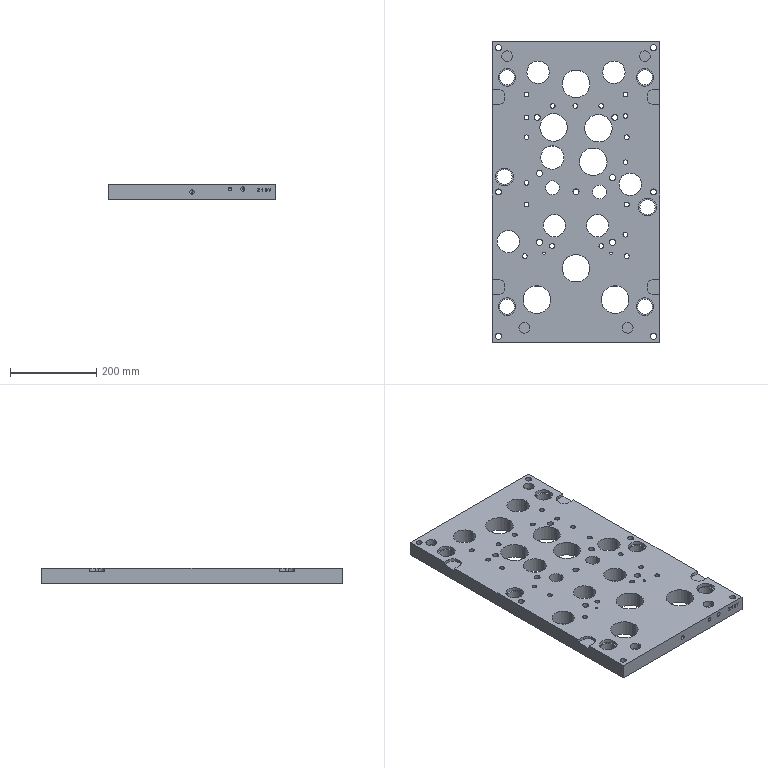Part | Creo | 1 solid | 404 faces | box 390 x 700 x 35 mm | volume 7700199 mm3 | cylinder 245 | plane 86 | cone 42 | other 31 | commonest cylinder face diameters 11 x36 18 x36 5.2 x30 14 x26 20 x26 64 x14